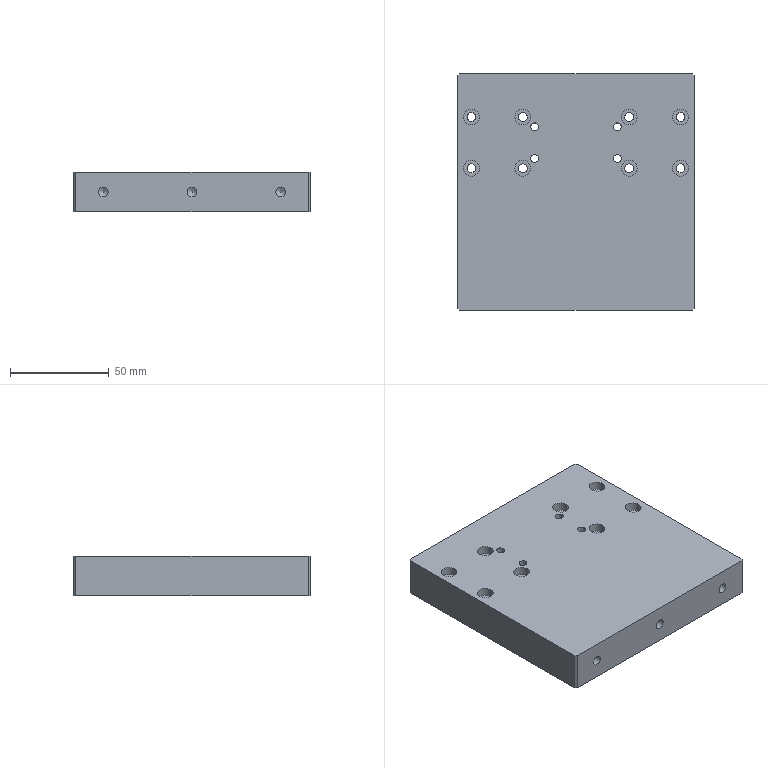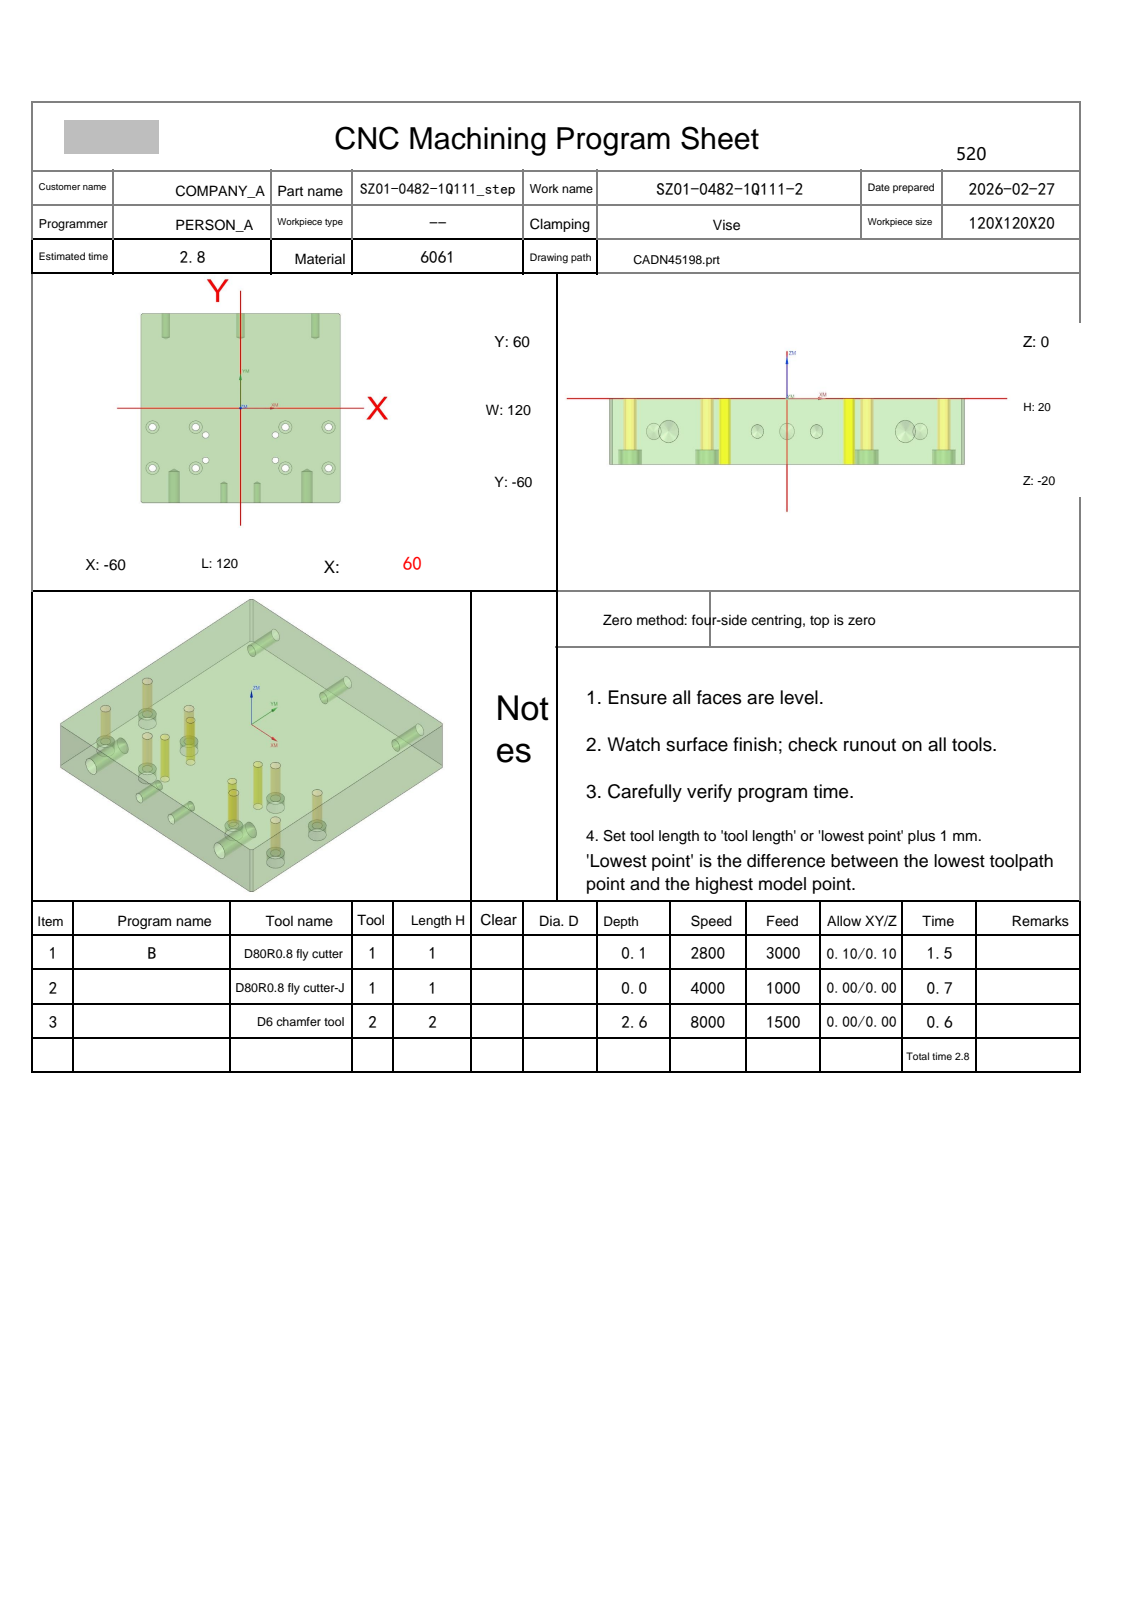NC program | NX | posted by the shop | part box 120 x 120 x 20 mm
Whole program:
%
O0001
(Machine time: 3.36 MIN)
(===Total Tool:2===)
(T1=D80R0.8 fly cutter D=80.  R=0.8  D-  H01 Z=0.    )
(T2=D6 chamfer tool   D=6.   R=0.   D-  H02 Z=-2.55 )
G80 G90 G17 G49 G40
G91 G28 Z0
M01
N1 T01 M06
(D80R0.8 fly cutter  D=80. R=0.8 H=01 ce=0.10 di=0.10)
G00 G90 G54 X112.097 Y-36.097 M03 S2800
G43 H01 Z50.
M08
Z6.011
G01 Z4.011 F3000.
X100.097
X-92.1
G02 X-100.097 Y-28.1 I.003 J8.
G01 Y20.74
G02 X-92.1 Y28.737 I8. J-.003
G01 X100.097
X112.097
Z6.011
G00 Y-36.097
Z5.522
G01 Z3.522
X100.097
X-92.1
G02 X-100.097 Y-28.1 I.003 J8.
G01 Y20.74
G02 X-92.1 Y28.737 I8. J-.003
G01 X100.097
X112.097
Z5.522
G00 Y-36.097
Z5.033
G01 Z3.033
X100.097
X-92.1
G02 X-100.097 Y-28.1 I.003 J8.
G01 Y20.74
G02 X-92.1 Y28.737 I8. J-.003
G01 X100.097
X112.097
Z5.033
G00 Y-36.097
Z4.544
G01 Z2.544
X100.097
X-92.1
G02 X-100.097 Y-28.1 I.003 J8.
G01 Y20.74
G02 X-92.1 Y28.737 I8. J-.003
G01 X100.097
X112.097
Z4.544
G00 Y-36.097
Z4.056
G01 Z2.056
X100.097
X-92.1
G02 X-100.097 Y-28.1 I.003 J8.
G01 Y20.74
G02 X-92.1 Y28.737 I8. J-.003
G01 X100.097
X112.097
Z4.056
G00 Y-36.097
Z3.567
G01 Z1.567
X100.097
X-92.1
G02 X-100.097 Y-28.1 I.003 J8.
G01 Y20.74
G02 X-92.1 Y28.737 I8. J-.003
G01 X100.097
X112.097
Z3.567
G00 Y-36.097
Z3.078
G01 Z1.078
X100.097
X-92.1
G02 X-100.097 Y-28.1 I.003 J8.
G01 Y20.74
G02 X-92.1 Y28.737 I8. J-.003
G01 X100.097
X112.097
Z3.078
G00 Y-36.097
Z2.589
G01 Z.589
X100.097
X-92.1
G02 X-100.097 Y-28.1 I.003 J8.
G01 Y20.74
G02 X-92.1 Y28.737 I8. J-.003
G01 X100.097
X112.097
Z2.589
G00 Y-36.097
Z2.1
G01 Z.1
X100.097
X-92.1
G02 X-100.097 Y-28.1 I.003 J8.
G01 Y20.74
G02 X-92.1 Y28.737 I8. J-.003
G01 X100.097
X112.097
Z2.1
G00 Z50.
G91 G28 Z0.0
M05
M09
G91 G28 Z0.0
M01
N2 T01 M06
(D80R0.8 fly cutter-J  D=80. R=0.8 H=01 ce=0.00 di=0.00)
G00 G90 G54 X111.999 Y-35.999 M03 S4000
G43 H01 Z50.
M08
Z2.
G01 Z0.0 F1000.
X99.999
X-92.799
G02 X-99.999 Y-28.799 I0.0 J7.2
G01 Y-11.68
G02 X-91.999 Y-3.68 I8. J0.0
G01 X92.799
G03 X99.999 Y3.52 I0.0 J7.2
G01 Y20.639
G03 X91.999 Y28.639 I-8. J0.0
G01 X-99.999
X-111.999
Z2.
G00 Z50.
G91 G28 Z0.0
M05
M09
G91 G28 Z0.0
M01
N3 T02 M06
(D6 chamfer tool  D=6. R=0. H=02 ce=0.00 di=0.00)
G00 G90 G54 X-21. Y-33. M03 S8000
G43 H02 Z50.
M08
G98 G81 X-21. Y-33. Z-2.3 R3. F1000.
Y-17.
X21.
Y-33.
G80
G00 Z50.
G00 G90 X53. Y-38. M03 S8000
Z50.
G98 G81 X53. Y-38. Z-2.55 R3. F1000.
Y-12.
X27.
Y-38.
X-27.
X-53.
Y-12.
X-27.
G80
G00 Z50.
G00 G90 X-61.227 Y-.386 M03 S6500
Z50.
Z.172
G01 Z-1.2 F1500.
G03 X-61.027 Y-.1 I-1.532 J1.286
G01 X-60.997 Y-.054
X-61. Y0.0
Y59.
X-60.966 Y59.259
X-60.866 Y59.5
X-60.707 Y59.707
X-59.707 Y60.707
X-59.5 Y60.866
X-59.259 Y60.966
X-59. Y61.
X59.
X59.259 Y60.966
X59.5 Y60.866
X59.707 Y60.707
X60.707 Y59.707
X60.866 Y59.5
X60.966 Y59.259
X61. Y59.
Y-59.
X60.966 Y-59.259
X60.866 Y-59.5
X60.707 Y-59.707
X59.707 Y-60.707
X59.5 Y-60.866
X59.259 Y-60.966
X59. Y-61.
X-59.
X-59.259 Y-60.966
X-59.5 Y-60.866
X-59.707 Y-60.707
X-60.707 Y-59.707
X-60.866 Y-59.5
X-60.966 Y-59.259
X-61. Y-59.
Y0.0
X-60.997 Y.054
X-61.027 Y.1
G03 X-61.227 Y.386 I-1.732 J-1.
G01 Z.172
G00 Z10.
X-54.065 Y-37.593
Z.294
G01 Z-1.2
G03 X-54.234 Y-37.898 I1.658 J-1.118
G01 X-54.259 Y-37.946
X-54.25 Y-38.
G03 X-53. Y-39.25 I1.25 J0.0
X-51.75 Y-38. I0.0 J1.25
X-53. Y-36.75 I-1.25 J0.0
X-54.223 Y-37.74 I0.0 J-1.25
G01 X-54.25 Y-38.
X-54.259 Y-38.054
X-54.234 Y-38.102
G03 X-54.065 Y-38.407 I1.827 J.813
G01 Z.294
G00 Z10.
Y-11.593
Z.294
G01 Z-1.2
G03 X-54.234 Y-11.898 I1.658 J-1.118
G01 X-54.259 Y-11.946
X-54.25 Y-12.
G03 X-53. Y-13.25 I1.25 J0.0
X-51.75 Y-12. I0.0 J1.25
X-53. Y-10.75 I-1.25 J0.0
X-54.223 Y-11.74 I0.0 J-1.25
G01 X-54.25 Y-12.
X-54.259 Y-12.054
X-54.234 Y-12.102
G03 X-54.065 Y-12.407 I1.827 J.813
G01 Z.294
G00 Z10.
X-28.065 Y-11.593
Z.294
G01 Z-1.2
G03 X-28.234 Y-11.898 I1.658 J-1.118
G01 X-28.259 Y-11.946
X-28.25 Y-12.
G03 X-27. Y-13.25 I1.25 J0.0
X-25.75 Y-12. I0.0 J1.25
X-27. Y-10.75 I-1.25 J0.0
X-28.223 Y-11.74 I0.0 J-1.25
G01 X-28.25 Y-12.
X-28.259 Y-12.054
X-28.234 Y-12.102
G03 X-28.065 Y-12.407 I1.827 J.813
G01 Z.294
G00 Z2.55
X-21.826 Y-16.588
Z.33
G01 Z-1.2
G03 X-21.986 Y-16.897 I1.687 J-1.075
G01 X-22.01 Y-16.946
X-22. Y-17.
G03 X-21. Y-18. I1. J0.0
X-20. Y-17. I0.0 J1.
X-21. Y-16. I-1. J0.0
X-22. Y-17. I0.0 J-1.
G01 X-22.01 Y-17.054
X-21.986 Y-17.103
G03 X-21.826 Y-17.412 I1.848 J.765
G01 Z.33
G00 Z10.
X-28.065 Y-37.593
Z.294
G01 Z-1.2
G03 X-28.234 Y-37.898 I1.658 J-1.118
G01 X-28.259 Y-37.946
X-28.25 Y-38.
G03 X-27. Y-39.25 I1.25 J0.0
X-25.75 Y-38. I0.0 J1.25
X-27. Y-36.75 I-1.25 J0.0
X-28.223 Y-37.74 I0.0 J-1.25
G01 X-28.25 Y-38.
X-28.259 Y-38.054
X-28.234 Y-38.102
G03 X-28.065 Y-38.407 I1.827 J.813
G01 Z.294
G00 Z2.55
X-21.826 Y-32.588
Z.33
G01 Z-1.2
G03 X-21.986 Y-32.897 I1.687 J-1.075
G01 X-22.01 Y-32.946
X-22. Y-33.
G03 X-21. Y-34. I1. J0.0
X-20. Y-33. I0.0 J1.
X-21. Y-32. I-1. J0.0
X-22. Y-33. I0.0 J-1.
G01 X-22.01 Y-33.054
X-21.986 Y-33.103
G03 X-21.826 Y-33.412 I1.848 J.765
G01 Z.33
G00 Z10.
X20.174 Y-32.588
Z.33
G01 Z-1.2
G03 X20.014 Y-32.897 I1.687 J-1.075
G01 X19.99 Y-32.946
X20. Y-33.
G03 X21. Y-34. I1. J0.0
X22. Y-33. I0.0 J1.
X21. Y-32. I-1. J0.0
X20. Y-33. I0.0 J-1.
G01 X19.99 Y-33.054
X20.014 Y-33.103
G03 X20.174 Y-33.412 I1.848 J.765
G01 Z.33
G00 Z2.55
X25.935 Y-37.593
Z.294
G01 Z-1.2
G03 X25.766 Y-37.898 I1.658 J-1.118
G01 X25.741 Y-37.946
X25.75 Y-38.
G03 X27. Y-39.25 I1.25 J0.0
X28.25 Y-38. I0.0 J1.25
X27. Y-36.75 I-1.25 J0.0
X25.777 Y-37.74 I0.0 J-1.25
G01 X25.75 Y-38.
X25.741 Y-38.054
X25.766 Y-38.102
G03 X25.935 Y-38.407 I1.827 J.813
G01 Z.294
G00 Z10.
X20.174 Y-16.588
Z.33
G01 Z-1.2
G03 X20.014 Y-16.897 I1.687 J-1.075
G01 X19.99 Y-16.946
X20. Y-17.
G03 X21. Y-18. I1. J0.0
X22. Y-17. I0.0 J1.
X21. Y-16. I-1. J0.0
X20. Y-17. I0.0 J-1.
G01 X19.99 Y-17.054
X20.014 Y-17.103
G03 X20.174 Y-17.412 I1.848 J.765
G01 Z.33
G00 Z2.55
X25.935 Y-11.593
Z.294
G01 Z-1.2
G03 X25.766 Y-11.898 I1.658 J-1.118
G01 X25.741 Y-11.946
X25.75 Y-12.
G03 X27. Y-13.25 I1.25 J0.0
X28.25 Y-12. I0.0 J1.25
X27. Y-10.75 I-1.25 J0.0
X25.777 Y-11.74 I0.0 J-1.25
G01 X25.75 Y-12.
X25.741 Y-12.054
X25.766 Y-12.102
G03 X25.935 Y-12.407 I1.827 J.813
G01 Z.294
G00 Z10.
X51.935 Y-11.593
Z.294
G01 Z-1.2
G03 X51.766 Y-11.898 I1.658 J-1.118
G01 X51.741 Y-11.946
X51.75 Y-12.
G03 X53. Y-13.25 I1.25 J0.0
X54.25 Y-12. I0.0 J1.25
X53. Y-10.75 I-1.25 J0.0
X51.777 Y-11.74 I0.0 J-1.25
G01 X51.75 Y-12.
X51.741 Y-12.054
X51.766 Y-12.102
G03 X51.935 Y-12.407 I1.827 J.813
G01 Z.294
G00 Z10.
Y-37.593
Z.294
G01 Z-1.2
G03 X51.766 Y-37.898 I1.658 J-1.118
G01 X51.741 Y-37.946
X51.75 Y-38.
G03 X53. Y-39.25 I1.25 J0.0
X54.25 Y-38. I0.0 J1.25
X53. Y-36.75 I-1.25 J0.0
X51.777 Y-37.74 I0.0 J-1.25
G01 X51.75 Y-38.
X51.741 Y-38.054
X51.766 Y-38.102
G03 X51.935 Y-38.407 I1.827 J.813
G01 Z.294
G00 Z50.
M05
M09
G91 G28 Z0.0
G91 G28 Y0.0
M30
%